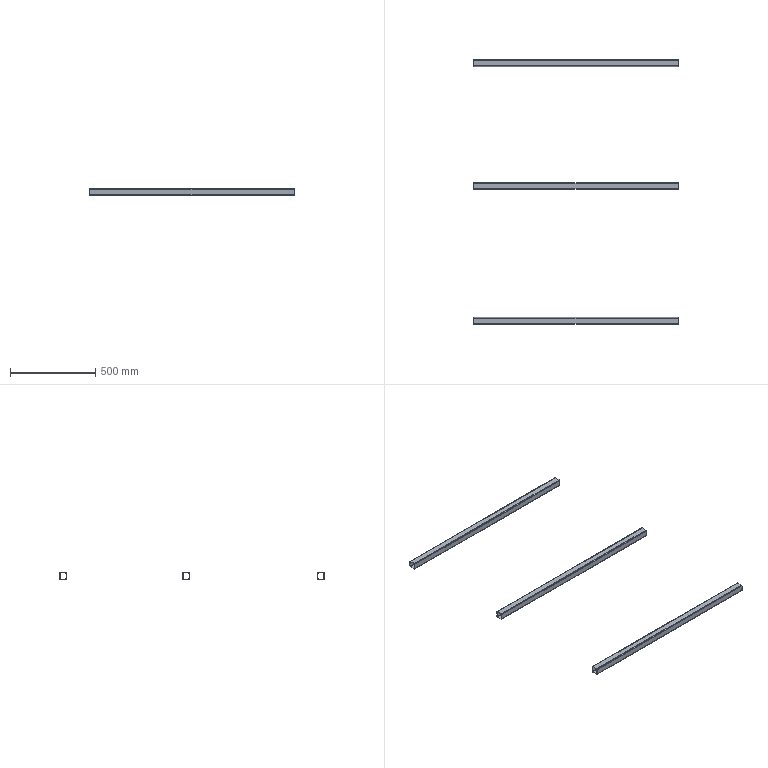Part | SolidWorks | features WeldMemberFeat 1, WeldmentFeature 1 | 3 solids | 54 faces | box 1200 x 1550 x 40 mm | volume 1199581 mm3 | plane 30 | cylinder 24 | commonest cylinder face diameters 4.6 x12 9.2 x12